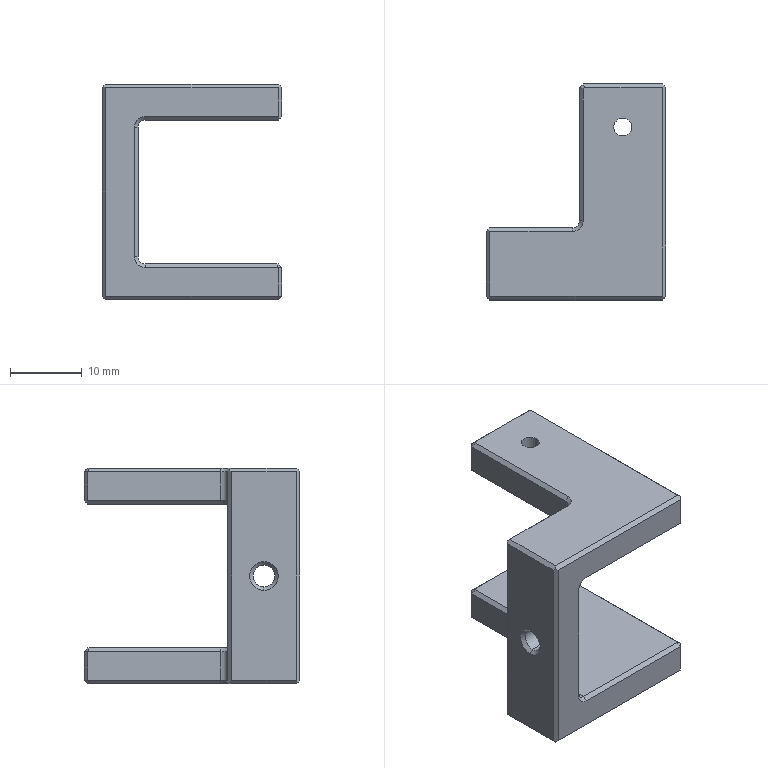Part | SolidWorks | features Chamfer 3, ICE 3, 3DProfileFeature 1, Extrusion 1, Fillet 1, HoleWzd 1 | 1 solid | 77 faces | box 25 x 30 x 30 mm | volume 5700 mm3 | plane 53 | cone 14 | cylinder 10 | commonest cylinder face diameters 2 x4 2.5 x2 3 x2 4.5 x2